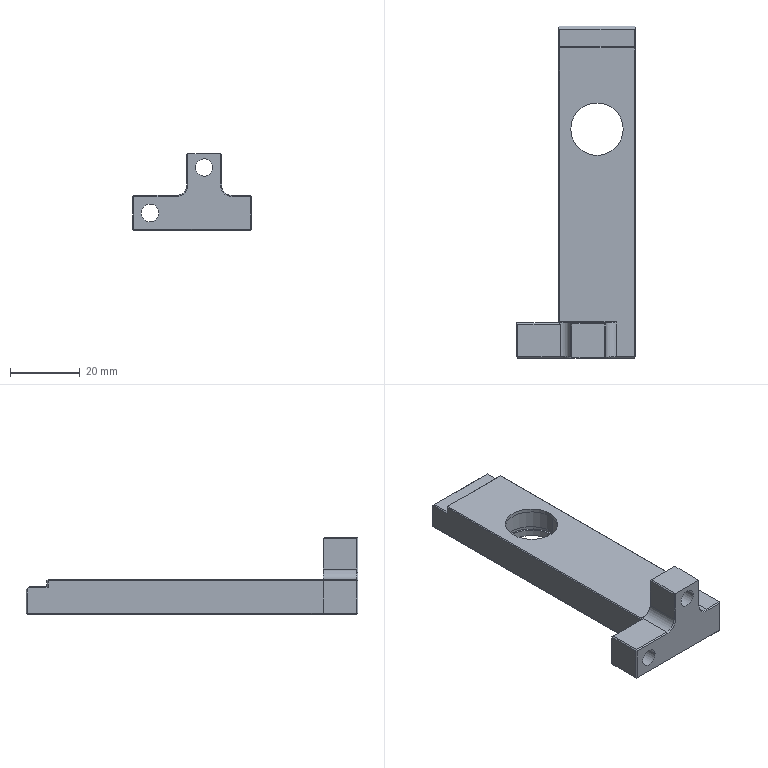Part | NX | features BREP 1 | 1 solid | 77 faces | box 34 x 95 x 22 mm | volume 20298 mm3 | plane 53 | cylinder 18 | cone 6 | commonest cylinder face diameters 2.5 x4 5 x4 17 x4 6 x2 15 x2 18 x2